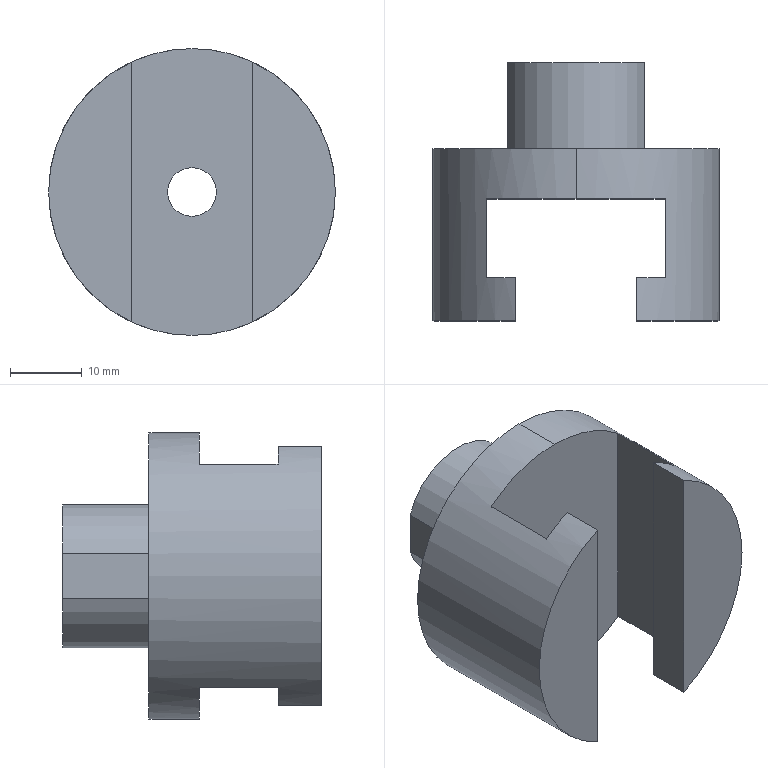Part | STEP file | union head A | 1 solid | 20 faces | box 40 x 36 x 40 mm | volume 19001 mm3 | plane 13 | cylinder 7 | commonest cylinder face diameters 20 x3 6.8 x2 40 x2
STEP:
#1=CARTESIAN_POINT('',(0.,0.,0.));
#2=DIRECTION('',(0.,0.,1.));
#3=DIRECTION('',(1.,0.,0.));
#4=AXIS2_PLACEMENT_3D('',#1,#2,#3);
#5=CARTESIAN_POINT('',(0.,17.,3.4));
#6=VERTEX_POINT('',#5);
#7=CARTESIAN_POINT('',(0.,36.,3.4));
#8=VERTEX_POINT('',#7);
#9=CARTESIAN_POINT('',(0.,36.,3.4));
#10=DIRECTION('',(0.,1.,0.));
#11=VECTOR('',#10,1.);
#12=LINE('',#9,#11);
#13=CARTESIAN_POINT('',(0.,36.,0.));
#14=DIRECTION('',(0.,1.,0.));
#15=DIRECTION('',(0.,0.,1.));
#16=AXIS2_PLACEMENT_3D('',#13,#14,#15);
#17=CYLINDRICAL_SURFACE('',#16,3.4);
#18=CARTESIAN_POINT('',(6.283,0.));
#19=DIRECTION('',(0.,1.));
#20=VECTOR('',#19,1.);
#21=LINE('',#18,#20);
#22=(GEOMETRIC_REPRESENTATION_CONTEXT(2)PARAMETRIC_REPRESENTATION_CONTEXT()REPRESENTATION_CONTEXT('',''));
#23=DEFINITIONAL_REPRESENTATION('',(#21),#22);
#24=PCURVE('',#17,#23);
#25=CARTESIAN_POINT('',(0.,36.,0.));
#26=DIRECTION('',(0.,1.,0.));
#27=DIRECTION('',(0.,0.,1.));
#28=AXIS2_PLACEMENT_3D('',#25,#26,#27);
#29=CYLINDRICAL_SURFACE('',#28,3.4);
#30=CARTESIAN_POINT('',(0.,0.));
#31=DIRECTION('',(0.,1.));
#32=VECTOR('',#31,1.);
#33=LINE('',#30,#32);
#34=(GEOMETRIC_REPRESENTATION_CONTEXT(2)PARAMETRIC_REPRESENTATION_CONTEXT()REPRESENTATION_CONTEXT('',''));
#35=DEFINITIONAL_REPRESENTATION('',(#33),#34);
#36=PCURVE('',#29,#35);
#37=SURFACE_CURVE('',#12,(#24,#36),.PCURVE_S1.);
#38=EDGE_CURVE('',#6,#8,#37,.T.);
#39=ORIENTED_EDGE('',*,*,#38,.T.);
#40=CARTESIAN_POINT('',(0.,36.,-3.4));
#41=VERTEX_POINT('',#40);
#42=CARTESIAN_POINT('',(0.,36.,0.));
#43=DIRECTION('',(0.,1.,0.));
#44=DIRECTION('',(0.,0.,1.));
#45=AXIS2_PLACEMENT_3D('',#42,#43,#44);
#46=CIRCLE('',#45,3.4);
#47=CARTESIAN_POINT('',(0.,0.));
#48=DIRECTION('',(1.,0.));
#49=VECTOR('',#48,1.);
#50=LINE('',#47,#49);
#51=(GEOMETRIC_REPRESENTATION_CONTEXT(2)PARAMETRIC_REPRESENTATION_CONTEXT()REPRESENTATION_CONTEXT('',''));
#52=DEFINITIONAL_REPRESENTATION('',(#50),#51);
#53=PCURVE('',#17,#52);
#54=CARTESIAN_POINT('',(0.,36.,0.));
#55=DIRECTION('',(0.,-1.,0.));
#56=DIRECTION('',(0.,0.,-1.));
#57=AXIS2_PLACEMENT_3D('',#54,#55,#56);
#58=PLANE('',#57);
#59=CARTESIAN_POINT('',(-3.4,0.));
#60=CARTESIAN_POINT('',(-3.4,5.889));
#61=CARTESIAN_POINT('',(1.7,2.944));
#62=CARTESIAN_POINT('',(6.8,0.));
#63=CARTESIAN_POINT('',(1.7,-2.944));
#64=CARTESIAN_POINT('',(-3.4,-5.889));
#65=CARTESIAN_POINT('',(-3.4,0.));
#66=(BOUNDED_CURVE()B_SPLINE_CURVE(2,(#59,#60,#61,#62,#63,#64,#65),.UNSPECIFIED.,.T.,.F.)B_SPLINE_CURVE_WITH_KNOTS((1,2,2,2,2,1),(-2.094,0.,2.094,4.189,6.283,8.378),.UNSPECIFIED.)CURVE()GEOMETRIC_REPRESENTATION_ITEM()RATIONAL_B_SPLINE_CURVE((1.,0.5,1.,0.5,1.,0.5,1.))REPRESENTATION_ITEM(''));
#67=(GEOMETRIC_REPRESENTATION_CONTEXT(2)PARAMETRIC_REPRESENTATION_CONTEXT()REPRESENTATION_CONTEXT('',''));
#68=DEFINITIONAL_REPRESENTATION('',(#66),#67);
#69=PCURVE('',#58,#68);
#70=SURFACE_CURVE('',#46,(#53,#69),.PCURVE_S1.);
#71=EDGE_CURVE('',#41,#8,#70,.T.);
#72=ORIENTED_EDGE('',*,*,#71,.F.);
#73=CARTESIAN_POINT('',(0.,17.,-3.4));
#74=VERTEX_POINT('',#73);
#75=CARTESIAN_POINT('',(0.,36.,-3.4));
#76=DIRECTION('',(0.,1.,0.));
#77=VECTOR('',#76,1.);
#78=LINE('',#75,#77);
#79=CARTESIAN_POINT('',(3.142,0.));
#80=DIRECTION('',(0.,1.));
#81=VECTOR('',#80,1.);
#82=LINE('',#79,#81);
#83=(GEOMETRIC_REPRESENTATION_CONTEXT(2)PARAMETRIC_REPRESENTATION_CONTEXT()REPRESENTATION_CONTEXT('',''));
#84=DEFINITIONAL_REPRESENTATION('',(#82),#83);
#85=PCURVE('',#17,#84);
#86=CARTESIAN_POINT('',(3.142,0.));
#87=DIRECTION('',(0.,1.));
#88=VECTOR('',#87,1.);
#89=LINE('',#86,#88);
#90=(GEOMETRIC_REPRESENTATION_CONTEXT(2)PARAMETRIC_REPRESENTATION_CONTEXT()REPRESENTATION_CONTEXT('',''));
#91=DEFINITIONAL_REPRESENTATION('',(#89),#90);
#92=PCURVE('',#29,#91);
#93=SURFACE_CURVE('',#78,(#85,#92),.PCURVE_S1.);
#94=EDGE_CURVE('',#74,#41,#93,.T.);
#95=ORIENTED_EDGE('',*,*,#94,.F.);
#96=CARTESIAN_POINT('',(0.,17.,0.));
#97=DIRECTION('',(0.,1.,0.));
#98=DIRECTION('',(0.,0.,1.));
#99=AXIS2_PLACEMENT_3D('',#96,#97,#98);
#100=CIRCLE('',#99,3.4);
#101=CARTESIAN_POINT('',(0.,-19.));
#102=DIRECTION('',(1.,0.));
#103=VECTOR('',#102,1.);
#104=LINE('',#101,#103);
#105=(GEOMETRIC_REPRESENTATION_CONTEXT(2)PARAMETRIC_REPRESENTATION_CONTEXT()REPRESENTATION_CONTEXT('',''));
#106=DEFINITIONAL_REPRESENTATION('',(#104),#105);
#107=PCURVE('',#17,#106);
#108=CARTESIAN_POINT('',(-12.5,17.,-20.));
#109=DIRECTION('',(0.,1.,0.));
#110=DIRECTION('',(0.,0.,1.));
#111=AXIS2_PLACEMENT_3D('',#108,#109,#110);
#112=PLANE('',#111);
#113=CARTESIAN_POINT('',(20.,12.5));
#114=DIRECTION('',(1.,0.));
#115=AXIS2_PLACEMENT_2D('',#113,#114);
#116=CIRCLE('',#115,3.4);
#117=(GEOMETRIC_REPRESENTATION_CONTEXT(2)PARAMETRIC_REPRESENTATION_CONTEXT()REPRESENTATION_CONTEXT('',''));
#118=DEFINITIONAL_REPRESENTATION('',(#116),#117);
#119=PCURVE('',#112,#118);
#120=SURFACE_CURVE('',#100,(#107,#119),.PCURVE_S1.);
#121=EDGE_CURVE('',#74,#6,#120,.T.);
#122=ORIENTED_EDGE('',*,*,#121,.T.);
#123=EDGE_LOOP('',(#39,#72,#95,#122));
#124=FACE_BOUND('',#123,.F.);
#125=ADVANCED_FACE('',(#124),#17,.F.);
#126=CARTESIAN_POINT('',(0.,24.,-20.));
#127=VERTEX_POINT('',#126);
#128=CARTESIAN_POINT('',(0.,24.,20.));
#129=VERTEX_POINT('',#128);
#130=CARTESIAN_POINT('',(0.,24.,0.));
#131=DIRECTION('',(0.,-1.,0.));
#132=DIRECTION('',(0.,0.,-1.));
#133=AXIS2_PLACEMENT_3D('',#130,#131,#132);
#134=CIRCLE('',#133,20.);
#135=CARTESIAN_POINT('',(0.,0.,0.));
#136=DIRECTION('',(0.,-1.,0.));
#137=DIRECTION('',(0.,0.,-1.));
#138=AXIS2_PLACEMENT_3D('',#135,#136,#137);
#139=CYLINDRICAL_SURFACE('',#138,20.);
#140=CARTESIAN_POINT('',(0.,-24.));
#141=DIRECTION('',(1.,0.));
#142=VECTOR('',#141,1.);
#143=LINE('',#140,#142);
#144=(GEOMETRIC_REPRESENTATION_CONTEXT(2)PARAMETRIC_REPRESENTATION_CONTEXT()REPRESENTATION_CONTEXT('',''));
#145=DEFINITIONAL_REPRESENTATION('',(#143),#144);
#146=PCURVE('',#139,#145);
#147=CARTESIAN_POINT('',(-10.,24.,0.));
#148=DIRECTION('',(0.,-1.,0.));
#149=DIRECTION('',(0.,0.,-1.));
#150=AXIS2_PLACEMENT_3D('',#147,#148,#149);
#151=PLANE('',#150);
#152=CARTESIAN_POINT('',(0.,10.));
#153=DIRECTION('',(1.,0.));
#154=AXIS2_PLACEMENT_2D('',#152,#153);
#155=CIRCLE('',#154,20.);
#156=(GEOMETRIC_REPRESENTATION_CONTEXT(2)PARAMETRIC_REPRESENTATION_CONTEXT()REPRESENTATION_CONTEXT('',''));
#157=DEFINITIONAL_REPRESENTATION('',(#155),#156);
#158=PCURVE('',#151,#157);
#159=SURFACE_CURVE('',#134,(#146,#158),.PCURVE_S1.);
#160=EDGE_CURVE('',#127,#129,#159,.T.);
#161=ORIENTED_EDGE('',*,*,#160,.T.);
#162=CARTESIAN_POINT('',(0.,17.,20.));
#163=VERTEX_POINT('',#162);
#164=CARTESIAN_POINT('',(0.,0.,20.));
#165=DIRECTION('',(0.,-1.,0.));
#166=VECTOR('',#165,1.);
#167=LINE('',#164,#166);
#168=CARTESIAN_POINT('',(3.142,0.));
#169=DIRECTION('',(0.,1.));
#170=VECTOR('',#169,1.);
#171=LINE('',#168,#170);
#172=(GEOMETRIC_REPRESENTATION_CONTEXT(2)PARAMETRIC_REPRESENTATION_CONTEXT()REPRESENTATION_CONTEXT('',''));
#173=DEFINITIONAL_REPRESENTATION('',(#171),#172);
#174=PCURVE('',#139,#173);
#175=CARTESIAN_POINT('',(0.,0.,0.));
#176=DIRECTION('',(0.,-1.,0.));
#177=DIRECTION('',(0.,0.,-1.));
#178=AXIS2_PLACEMENT_3D('',#175,#176,#177);
#179=CYLINDRICAL_SURFACE('',#178,20.);
#180=CARTESIAN_POINT('',(3.142,0.));
#181=DIRECTION('',(0.,1.));
#182=VECTOR('',#181,1.);
#183=LINE('',#180,#182);
#184=(GEOMETRIC_REPRESENTATION_CONTEXT(2)PARAMETRIC_REPRESENTATION_CONTEXT()REPRESENTATION_CONTEXT('',''));
#185=DEFINITIONAL_REPRESENTATION('',(#183),#184);
#186=PCURVE('',#179,#185);
#187=SURFACE_CURVE('',#167,(#174,#186),.PCURVE_S1.);
#188=EDGE_CURVE('',#129,#163,#187,.T.);
#189=ORIENTED_EDGE('',*,*,#188,.T.);
#190=CARTESIAN_POINT('',(12.5,17.,15.612));
#191=VERTEX_POINT('',#190);
#192=CARTESIAN_POINT('',(0.,17.,0.));
#193=DIRECTION('',(0.,1.,0.));
#194=DIRECTION('',(0.,0.,1.));
#195=AXIS2_PLACEMENT_3D('',#192,#193,#194);
#196=CIRCLE('',#195,20.);
#197=CARTESIAN_POINT('',(3.142,-17.));
#198=DIRECTION('',(-1.,0.));
#199=VECTOR('',#198,1.);
#200=LINE('',#197,#199);
#201=(GEOMETRIC_REPRESENTATION_CONTEXT(2)PARAMETRIC_REPRESENTATION_CONTEXT()REPRESENTATION_CONTEXT('',''));
#202=DEFINITIONAL_REPRESENTATION('',(#200),#201);
#203=PCURVE('',#139,#202);
#204=CARTESIAN_POINT('',(20.,12.5));
#205=DIRECTION('',(1.,0.));
#206=AXIS2_PLACEMENT_2D('',#204,#205);
#207=CIRCLE('',#206,20.);
#208=(GEOMETRIC_REPRESENTATION_CONTEXT(2)PARAMETRIC_REPRESENTATION_CONTEXT()REPRESENTATION_CONTEXT('',''));
#209=DEFINITIONAL_REPRESENTATION('',(#207),#208);
#210=PCURVE('',#112,#209);
#211=SURFACE_CURVE('',#196,(#203,#210),.PCURVE_S1.);
#212=EDGE_CURVE('',#163,#191,#211,.T.);
#213=ORIENTED_EDGE('',*,*,#212,.T.);
#214=CARTESIAN_POINT('',(12.5,6.,15.612));
#215=VERTEX_POINT('',#214);
#216=CARTESIAN_POINT('',(12.5,0.,15.612));
#217=DIRECTION('',(0.,-1.,0.));
#218=VECTOR('',#217,1.);
#219=LINE('',#216,#218);
#220=CARTESIAN_POINT('',(2.466,0.));
#221=DIRECTION('',(0.,1.));
#222=VECTOR('',#221,1.);
#223=LINE('',#220,#222);
#224=(GEOMETRIC_REPRESENTATION_CONTEXT(2)PARAMETRIC_REPRESENTATION_CONTEXT()REPRESENTATION_CONTEXT('',''));
#225=DEFINITIONAL_REPRESENTATION('',(#223),#224);
#226=PCURVE('',#139,#225);
#227=CARTESIAN_POINT('',(12.5,17.,-20.));
#228=DIRECTION('',(1.,0.,0.));
#229=DIRECTION('',(0.,1.,0.));
#230=AXIS2_PLACEMENT_3D('',#227,#228,#229);
#231=PLANE('',#230);
#232=CARTESIAN_POINT('',(-17.,35.612));
#233=DIRECTION('',(-1.,0.));
#234=VECTOR('',#233,1.);
#235=LINE('',#232,#234);
#236=(GEOMETRIC_REPRESENTATION_CONTEXT(2)PARAMETRIC_REPRESENTATION_CONTEXT()REPRESENTATION_CONTEXT('',''));
#237=DEFINITIONAL_REPRESENTATION('',(#235),#236);
#238=PCURVE('',#231,#237);
#239=SURFACE_CURVE('',#219,(#226,#238),.PCURVE_S1.);
#240=EDGE_CURVE('',#191,#215,#239,.T.);
#241=ORIENTED_EDGE('',*,*,#240,.T.);
#242=CARTESIAN_POINT('',(8.5,6.,18.104));
#243=VERTEX_POINT('',#242);
#244=CARTESIAN_POINT('',(0.,6.,0.));
#245=DIRECTION('',(0.,-1.,0.));
#246=DIRECTION('',(0.,0.,-1.));
#247=AXIS2_PLACEMENT_3D('',#244,#245,#246);
#248=CIRCLE('',#247,20.);
#249=CARTESIAN_POINT('',(0.,-6.));
#250=DIRECTION('',(1.,0.));
#251=VECTOR('',#250,1.);
#252=LINE('',#249,#251);
#253=(GEOMETRIC_REPRESENTATION_CONTEXT(2)PARAMETRIC_REPRESENTATION_CONTEXT()REPRESENTATION_CONTEXT('',''));
#254=DEFINITIONAL_REPRESENTATION('',(#252),#253);
#255=PCURVE('',#139,#254);
#256=CARTESIAN_POINT('',(8.5,6.,-20.));
#257=DIRECTION('',(0.,-1.,0.));
#258=DIRECTION('',(0.,0.,-1.));
#259=AXIS2_PLACEMENT_3D('',#256,#257,#258);
#260=PLANE('',#259);
#261=CARTESIAN_POINT('',(-20.,-8.5));
#262=DIRECTION('',(1.,0.));
#263=AXIS2_PLACEMENT_2D('',#261,#262);
#264=CIRCLE('',#263,20.);
#265=(GEOMETRIC_REPRESENTATION_CONTEXT(2)PARAMETRIC_REPRESENTATION_CONTEXT()REPRESENTATION_CONTEXT('',''));
#266=DEFINITIONAL_REPRESENTATION('',(#264),#265);
#267=PCURVE('',#260,#266);
#268=SURFACE_CURVE('',#248,(#255,#267),.PCURVE_S1.);
#269=EDGE_CURVE('',#215,#243,#268,.T.);
#270=ORIENTED_EDGE('',*,*,#269,.T.);
#271=CARTESIAN_POINT('',(8.5,0.,18.104));
#272=VERTEX_POINT('',#271);
#273=CARTESIAN_POINT('',(8.5,0.,18.104));
#274=DIRECTION('',(0.,-1.,0.));
#275=VECTOR('',#274,1.);
#276=LINE('',#273,#275);
#277=CARTESIAN_POINT('',(2.703,0.));
#278=DIRECTION('',(0.,1.));
#279=VECTOR('',#278,1.);
#280=LINE('',#277,#279);
#281=(GEOMETRIC_REPRESENTATION_CONTEXT(2)PARAMETRIC_REPRESENTATION_CONTEXT()REPRESENTATION_CONTEXT('',''));
#282=DEFINITIONAL_REPRESENTATION('',(#280),#281);
#283=PCURVE('',#139,#282);
#284=CARTESIAN_POINT('',(8.5,0.,-20.));
#285=DIRECTION('',(1.,0.,0.));
#286=DIRECTION('',(0.,0.,-1.));
#287=AXIS2_PLACEMENT_3D('',#284,#285,#286);
#288=PLANE('',#287);
#289=CARTESIAN_POINT('',(-38.104,0.));
#290=DIRECTION('',(0.,-1.));
#291=VECTOR('',#290,1.);
#292=LINE('',#289,#291);
#293=(GEOMETRIC_REPRESENTATION_CONTEXT(2)PARAMETRIC_REPRESENTATION_CONTEXT()REPRESENTATION_CONTEXT('',''));
#294=DEFINITIONAL_REPRESENTATION('',(#292),#293);
#295=PCURVE('',#288,#294);
#296=SURFACE_CURVE('',#276,(#283,#295),.PCURVE_S1.);
#297=EDGE_CURVE('',#243,#272,#296,.T.);
#298=ORIENTED_EDGE('',*,*,#297,.T.);
#299=CARTESIAN_POINT('',(8.5,0.,-18.104));
#300=VERTEX_POINT('',#299);
#301=CARTESIAN_POINT('',(0.,0.,0.));
#302=DIRECTION('',(0.,-1.,0.));
#303=DIRECTION('',(0.,0.,-1.));
#304=AXIS2_PLACEMENT_3D('',#301,#302,#303);
#305=CIRCLE('',#304,20.);
#306=CARTESIAN_POINT('',(0.,0.));
#307=DIRECTION('',(1.,0.));
#308=VECTOR('',#307,1.);
#309=LINE('',#306,#308);
#310=(GEOMETRIC_REPRESENTATION_CONTEXT(2)PARAMETRIC_REPRESENTATION_CONTEXT()REPRESENTATION_CONTEXT('',''));
#311=DEFINITIONAL_REPRESENTATION('',(#309),#310);
#312=PCURVE('',#139,#311);
#313=CARTESIAN_POINT('',(-20.,0.,0.));
#314=DIRECTION('',(0.,1.,0.));
#315=DIRECTION('',(0.,0.,1.));
#316=AXIS2_PLACEMENT_3D('',#313,#314,#315);
#317=PLANE('',#316);
#318=CARTESIAN_POINT('',(-20.,20.));
#319=CARTESIAN_POINT('',(-20.,54.641));
#320=CARTESIAN_POINT('',(10.,37.321));
#321=CARTESIAN_POINT('',(40.,20.));
#322=CARTESIAN_POINT('',(10.,2.679));
#323=CARTESIAN_POINT('',(-20.,-14.641));
#324=CARTESIAN_POINT('',(-20.,20.));
#325=(BOUNDED_CURVE()B_SPLINE_CURVE(2,(#318,#319,#320,#321,#322,#323,#324),.UNSPECIFIED.,.T.,.F.)B_SPLINE_CURVE_WITH_KNOTS((1,2,2,2,2,1),(-2.094,0.,2.094,4.189,6.283,8.378),.UNSPECIFIED.)CURVE()GEOMETRIC_REPRESENTATION_ITEM()RATIONAL_B_SPLINE_CURVE((1.,0.5,1.,0.5,1.,0.5,1.))REPRESENTATION_ITEM(''));
#326=(GEOMETRIC_REPRESENTATION_CONTEXT(2)PARAMETRIC_REPRESENTATION_CONTEXT()REPRESENTATION_CONTEXT('',''));
#327=DEFINITIONAL_REPRESENTATION('',(#325),#326);
#328=PCURVE('',#317,#327);
#329=SURFACE_CURVE('',#305,(#312,#328),.PCURVE_S1.);
#330=EDGE_CURVE('',#300,#272,#329,.T.);
#331=ORIENTED_EDGE('',*,*,#330,.F.);
#332=CARTESIAN_POINT('',(8.5,6.,-18.104));
#333=VERTEX_POINT('',#332);
#334=CARTESIAN_POINT('',(8.5,0.,-18.104));
#335=DIRECTION('',(0.,1.,0.));
#336=VECTOR('',#335,1.);
#337=LINE('',#334,#336);
#338=CARTESIAN_POINT('',(0.439,0.));
#339=DIRECTION('',(0.,-1.));
#340=VECTOR('',#339,1.);
#341=LINE('',#338,#340);
#342=(GEOMETRIC_REPRESENTATION_CONTEXT(2)PARAMETRIC_REPRESENTATION_CONTEXT()REPRESENTATION_CONTEXT('',''));
#343=DEFINITIONAL_REPRESENTATION('',(#341),#342);
#344=PCURVE('',#139,#343);
#345=CARTESIAN_POINT('',(-1.896,0.));
#346=DIRECTION('',(0.,1.));
#347=VECTOR('',#346,1.);
#348=LINE('',#345,#347);
#349=(GEOMETRIC_REPRESENTATION_CONTEXT(2)PARAMETRIC_REPRESENTATION_CONTEXT()REPRESENTATION_CONTEXT('',''));
#350=DEFINITIONAL_REPRESENTATION('',(#348),#349);
#351=PCURVE('',#288,#350);
#352=SURFACE_CURVE('',#337,(#344,#351),.PCURVE_S1.);
#353=EDGE_CURVE('',#300,#333,#352,.T.);
#354=ORIENTED_EDGE('',*,*,#353,.T.);
#355=CARTESIAN_POINT('',(12.5,6.,-15.612));
#356=VERTEX_POINT('',#355);
#357=CARTESIAN_POINT('',(0.,6.,0.));
#358=DIRECTION('',(0.,-1.,0.));
#359=DIRECTION('',(0.,0.,-1.));
#360=AXIS2_PLACEMENT_3D('',#357,#358,#359);
#361=CIRCLE('',#360,20.);
#362=CARTESIAN_POINT('',(0.,-6.));
#363=DIRECTION('',(1.,0.));
#364=VECTOR('',#363,1.);
#365=LINE('',#362,#364);
#366=(GEOMETRIC_REPRESENTATION_CONTEXT(2)PARAMETRIC_REPRESENTATION_CONTEXT()REPRESENTATION_CONTEXT('',''));
#367=DEFINITIONAL_REPRESENTATION('',(#365),#366);
#368=PCURVE('',#139,#367);
#369=CARTESIAN_POINT('',(-20.,-8.5));
#370=DIRECTION('',(1.,0.));
#371=AXIS2_PLACEMENT_2D('',#369,#370);
#372=CIRCLE('',#371,20.);
#373=(GEOMETRIC_REPRESENTATION_CONTEXT(2)PARAMETRIC_REPRESENTATION_CONTEXT()REPRESENTATION_CONTEXT('',''));
#374=DEFINITIONAL_REPRESENTATION('',(#372),#373);
#375=PCURVE('',#260,#374);
#376=SURFACE_CURVE('',#361,(#368,#375),.PCURVE_S1.);
#377=EDGE_CURVE('',#333,#356,#376,.T.);
#378=ORIENTED_EDGE('',*,*,#377,.T.);
#379=CARTESIAN_POINT('',(12.5,17.,-15.612));
#380=VERTEX_POINT('',#379);
#381=CARTESIAN_POINT('',(12.5,0.,-15.612));
#382=DIRECTION('',(0.,1.,0.));
#383=VECTOR('',#382,1.);
#384=LINE('',#381,#383);
#385=CARTESIAN_POINT('',(0.6751,0.));
#386=DIRECTION('',(0.,-1.));
#387=VECTOR('',#386,1.);
#388=LINE('',#385,#387);
#389=(GEOMETRIC_REPRESENTATION_CONTEXT(2)PARAMETRIC_REPRESENTATION_CONTEXT()REPRESENTATION_CONTEXT('',''));
#390=DEFINITIONAL_REPRESENTATION('',(#388),#389);
#391=PCURVE('',#139,#390);
#392=CARTESIAN_POINT('',(-17.,4.388));
#393=DIRECTION('',(1.,0.));
#394=VECTOR('',#393,1.);
#395=LINE('',#392,#394);
#396=(GEOMETRIC_REPRESENTATION_CONTEXT(2)PARAMETRIC_REPRESENTATION_CONTEXT()REPRESENTATION_CONTEXT('',''));
#397=DEFINITIONAL_REPRESENTATION('',(#395),#396);
#398=PCURVE('',#231,#397);
#399=SURFACE_CURVE('',#384,(#391,#398),.PCURVE_S1.);
#400=EDGE_CURVE('',#356,#380,#399,.T.);
#401=ORIENTED_EDGE('',*,*,#400,.T.);
#402=CARTESIAN_POINT('',(0.,17.,-20.));
#403=VERTEX_POINT('',#402);
#404=CARTESIAN_POINT('',(0.,17.,0.));
#405=DIRECTION('',(0.,1.,0.));
#406=DIRECTION('',(0.,0.,1.));
#407=AXIS2_PLACEMENT_3D('',#404,#405,#406);
#408=CIRCLE('',#407,20.);
#409=CARTESIAN_POINT('',(3.142,-17.));
#410=DIRECTION('',(-1.,0.));
#411=VECTOR('',#410,1.);
#412=LINE('',#409,#411);
#413=(GEOMETRIC_REPRESENTATION_CONTEXT(2)PARAMETRIC_REPRESENTATION_CONTEXT()REPRESENTATION_CONTEXT('',''));
#414=DEFINITIONAL_REPRESENTATION('',(#412),#413);
#415=PCURVE('',#139,#414);
#416=CARTESIAN_POINT('',(20.,12.5));
#417=DIRECTION('',(1.,0.));
#418=AXIS2_PLACEMENT_2D('',#416,#417);
#419=CIRCLE('',#418,20.);
#420=(GEOMETRIC_REPRESENTATION_CONTEXT(2)PARAMETRIC_REPRESENTATION_CONTEXT()REPRESENTATION_CONTEXT('',''));
#421=DEFINITIONAL_REPRESENTATION('',(#419),#420);
#422=PCURVE('',#112,#421);
#423=SURFACE_CURVE('',#408,(#415,#422),.PCURVE_S1.);
#424=EDGE_CURVE('',#380,#403,#423,.T.);
#425=ORIENTED_EDGE('',*,*,#424,.T.);
#426=CARTESIAN_POINT('',(0.,0.,-20.));
#427=DIRECTION('',(0.,-1.,0.));
#428=VECTOR('',#427,1.);
#429=LINE('',#426,#428);
#430=CARTESIAN_POINT('',(0.,0.));
#431=DIRECTION('',(0.,1.));
#432=VECTOR('',#431,1.);
#433=LINE('',#430,#432);
#434=(GEOMETRIC_REPRESENTATION_CONTEXT(2)PARAMETRIC_REPRESENTATION_CONTEXT()REPRESENTATION_CONTEXT('',''));
#435=DEFINITIONAL_REPRESENTATION('',(#433),#434);
#436=PCURVE('',#139,#435);
#437=CARTESIAN_POINT('',(6.283,0.));
#438=DIRECTION('',(0.,1.));
#439=VECTOR('',#438,1.);
#440=LINE('',#437,#439);
#441=(GEOMETRIC_REPRESENTATION_CONTEXT(2)PARAMETRIC_REPRESENTATION_CONTEXT()REPRESENTATION_CONTEXT('',''));
#442=DEFINITIONAL_REPRESENTATION('',(#440),#441);
#443=PCURVE('',#179,#442);
#444=SURFACE_CURVE('',#429,(#436,#443),.PCURVE_S1.);
#445=EDGE_CURVE('',#127,#403,#444,.T.);
#446=ORIENTED_EDGE('',*,*,#445,.F.);
#447=EDGE_LOOP('',(#161,#189,#213,#241,#270,#298,#331,#354,#378,#401,#425,#446));
#448=FACE_BOUND('',#447,.T.);
#449=ADVANCED_FACE('',(#448),#139,.T.);
#450=CARTESIAN_POINT('',(-9.5,36.,-3.122));
#451=VERTEX_POINT('',#450);
#452=CARTESIAN_POINT('',(0.,36.,-10.));
#453=VERTEX_POINT('',#452);
#454=CARTESIAN_POINT('',(0.,36.,0.));
#455=DIRECTION('',(0.,-1.,0.));
#456=DIRECTION('',(0.,0.,-1.));
#457=AXIS2_PLACEMENT_3D('',#454,#455,#456);
#458=CIRCLE('',#457,10.);
#459=CARTESIAN_POINT('',(0.,0.,0.));
#460=DIRECTION('',(0.,-1.,0.));
#461=DIRECTION('',(0.,0.,-1.));
#462=AXIS2_PLACEMENT_3D('',#459,#460,#461);
#463=CYLINDRICAL_SURFACE('',#462,10.);
#464=CARTESIAN_POINT('',(0.,-36.));
#465=DIRECTION('',(1.,0.));
#466=VECTOR('',#465,1.);
#467=LINE('',#464,#466);
#468=(GEOMETRIC_REPRESENTATION_CONTEXT(2)PARAMETRIC_REPRESENTATION_CONTEXT()REPRESENTATION_CONTEXT('',''));
#469=DEFINITIONAL_REPRESENTATION('',(#467),#468);
#470=PCURVE('',#463,#469);
#471=CARTESIAN_POINT('',(0.,0.));
#472=DIRECTION('',(1.,0.));
#473=AXIS2_PLACEMENT_2D('',#471,#472);
#474=CIRCLE('',#473,10.);
#475=(GEOMETRIC_REPRESENTATION_CONTEXT(2)PARAMETRIC_REPRESENTATION_CONTEXT()REPRESENTATION_CONTEXT('',''));
#476=DEFINITIONAL_REPRESENTATION('',(#474),#475);
#477=PCURVE('',#58,#476);
#478=SURFACE_CURVE('',#458,(#470,#477),.PCURVE_S1.);
#479=EDGE_CURVE('',#451,#453,#478,.T.);
#480=ORIENTED_EDGE('',*,*,#479,.T.);
#481=CARTESIAN_POINT('',(0.,24.,-10.));
#482=VERTEX_POINT('',#481);
#483=CARTESIAN_POINT('',(0.,0.,-10.));
#484=DIRECTION('',(0.,-1.,0.));
#485=VECTOR('',#484,1.);
#486=LINE('',#483,#485);
#487=CARTESIAN_POINT('',(6.283,0.));
#488=DIRECTION('',(0.,1.));
#489=VECTOR('',#488,1.);
#490=LINE('',#487,#489);
#491=(GEOMETRIC_REPRESENTATION_CONTEXT(2)PARAMETRIC_REPRESENTATION_CONTEXT()REPRESENTATION_CONTEXT('',''));
#492=DEFINITIONAL_REPRESENTATION('',(#490),#491);
#493=PCURVE('',#463,#492);
#494=CARTESIAN_POINT('',(0.,0.,0.));
#495=DIRECTION('',(0.,-1.,0.));
#496=DIRECTION('',(0.,0.,-1.));
#497=AXIS2_PLACEMENT_3D('',#494,#495,#496);
#498=CYLINDRICAL_SURFACE('',#497,10.);
#499=CARTESIAN_POINT('',(0.,0.));
#500=DIRECTION('',(0.,1.));
#501=VECTOR('',#500,1.);
#502=LINE('',#499,#501);
#503=(GEOMETRIC_REPRESENTATION_CONTEXT(2)PARAMETRIC_REPRESENTATION_CONTEXT()REPRESENTATION_CONTEXT('',''));
#504=DEFINITIONAL_REPRESENTATION('',(#502),#503);
#505=PCURVE('',#498,#504);
#506=SURFACE_CURVE('',#486,(#493,#505),.PCURVE_S1.);
#507=EDGE_CURVE('',#453,#482,#506,.T.);
#508=ORIENTED_EDGE('',*,*,#507,.T.);
#509=CARTESIAN_POINT('',(-9.5,24.,-3.122));
#510=VERTEX_POINT('',#509);
#511=CARTESIAN_POINT('',(0.,24.,0.));
#512=DIRECTION('',(0.,-1.,0.));
#513=DIRECTION('',(0.,0.,-1.));
#514=AXIS2_PLACEMENT_3D('',#511,#512,#513);
#515=CIRCLE('',#514,10.);
#516=CARTESIAN_POINT('',(0.,-24.));
#517=DIRECTION('',(1.,0.));
#518=VECTOR('',#517,1.);
#519=LINE('',#516,#518);
#520=(GEOMETRIC_REPRESENTATION_CONTEXT(2)PARAMETRIC_REPRESENTATION_CONTEXT()REPRESENTATION_CONTEXT('',''));
#521=DEFINITIONAL_REPRESENTATION('',(#519),#520);
#522=PCURVE('',#463,#521);
#523=CARTESIAN_POINT('',(0.,10.));
#524=DIRECTION('',(1.,0.));
#525=AXIS2_PLACEMENT_2D('',#523,#524);
#526=CIRCLE('',#525,10.);
#527=(GEOMETRIC_REPRESENTATION_CONTEXT(2)PARAMETRIC_REPRESENTATION_CONTEXT()REPRESENTATION_CONTEXT('',''));
#528=DEFINITIONAL_REPRESENTATION('',(#526),#527);
#529=PCURVE('',#151,#528);
#530=SURFACE_CURVE('',#515,(#522,#529),.PCURVE_S1.);
#531=EDGE_CURVE('',#510,#482,#530,.T.);
#532=ORIENTED_EDGE('',*,*,#531,.F.);
#533=CARTESIAN_POINT('',(-9.5,0.,-3.122));
#534=DIRECTION('',(0.,1.,0.));
#535=VECTOR('',#534,1.);
#536=LINE('',#533,#535);
#537=CARTESIAN_POINT('',(5.03,0.));
#538=DIRECTION('',(0.,-1.));
#539=VECTOR('',#538,1.);
#540=LINE('',#537,#539);
#541=(GEOMETRIC_REPRESENTATION_CONTEXT(2)PARAMETRIC_REPRESENTATION_CONTEXT()REPRESENTATION_CONTEXT('',''));
#542=DEFINITIONAL_REPRESENTATION('',(#540),#541);
#543=PCURVE('',#463,#542);
#544=CARTESIAN_POINT('',(-9.5,6.26,-6.601));
#545=DIRECTION('',(1.,0.,0.));
#546=DIRECTION('',(0.,0.,-1.));
#547=AXIS2_PLACEMENT_3D('',#544,#545,#546);
#548=PLANE('',#547);
#549=CARTESIAN_POINT('',(-3.479,-6.26));
#550=DIRECTION('',(0.,1.));
#551=VECTOR('',#550,1.);
#552=LINE('',#549,#551);
#553=(GEOMETRIC_REPRESENTATION_CONTEXT(2)PARAMETRIC_REPRESENTATION_CONTEXT()REPRESENTATION_CONTEXT('',''));
#554=DEFINITIONAL_REPRESENTATION('',(#552),#553);
#555=PCURVE('',#548,#554);
#556=SURFACE_CURVE('',#536,(#543,#555),.PCURVE_S1.);
#557=EDGE_CURVE('',#510,#451,#556,.T.);
#558=ORIENTED_EDGE('',*,*,#557,.T.);
#559=EDGE_LOOP('',(#480,#508,#532,#558));
#560=FACE_BOUND('',#559,.T.);
#561=ADVANCED_FACE('',(#560),#463,.T.);
#562=CARTESIAN_POINT('',(-8.5,0.,18.104));
#563=VERTEX_POINT('',#562);
#564=CARTESIAN_POINT('',(-8.5,0.,-18.104));
#565=VERTEX_POINT('',#564);
#566=CARTESIAN_POINT('',(0.,0.,0.));
#567=DIRECTION('',(0.,-1.,0.));
#568=DIRECTION('',(0.,0.,-1.));
#569=AXIS2_PLACEMENT_3D('',#566,#567,#568);
#570=CIRCLE('',#569,20.);
#571=CARTESIAN_POINT('',(-20.,0.,0.));
#572=DIRECTION('',(0.,1.,0.));
#573=DIRECTION('',(0.,0.,1.));
#574=AXIS2_PLACEMENT_3D('',#571,#572,#573);
#575=PLANE('',#574);
#576=CARTESIAN_POINT('',(-20.,20.));
#577=CARTESIAN_POINT('',(-20.,54.641));
#578=CARTESIAN_POINT('',(10.,37.321));
#579=CARTESIAN_POINT('',(40.,20.));
#580=CARTESIAN_POINT('',(10.,2.679));
#581=CARTESIAN_POINT('',(-20.,-14.641));
#582=CARTESIAN_POINT('',(-20.,20.));
#583=(BOUNDED_CURVE()B_SPLINE_CURVE(2,(#576,#577,#578,#579,#580,#581,#582),.UNSPECIFIED.,.T.,.F.)B_SPLINE_CURVE_WITH_KNOTS((1,2,2,2,2,1),(-2.094,0.,2.094,4.189,6.283,8.378),.UNSPECIFIED.)CURVE()GEOMETRIC_REPRESENTATION_ITEM()RATIONAL_B_SPLINE_CURVE((1.,0.5,1.,0.5,1.,0.5,1.))REPRESENTATION_ITEM(''));
#584=(GEOMETRIC_REPRESENTATION_CONTEXT(2)PARAMETRIC_REPRESENTATION_CONTEXT()REPRESENTATION_CONTEXT('',''));
#585=DEFINITIONAL_REPRESENTATION('',(#583),#584);
#586=PCURVE('',#575,#585);
#587=CARTESIAN_POINT('',(0.,0.));
#588=DIRECTION('',(1.,0.));
#589=VECTOR('',#588,1.);
#590=LINE('',#587,#589);
#591=(GEOMETRIC_REPRESENTATION_CONTEXT(2)PARAMETRIC_REPRESENTATION_CONTEXT()REPRESENTATION_CONTEXT('',''));
#592=DEFINITIONAL_REPRESENTATION('',(#590),#591);
#593=PCURVE('',#179,#592);
#594=SURFACE_CURVE('',#570,(#586,#593),.PCURVE_S1.);
#595=EDGE_CURVE('',#563,#565,#594,.T.);
#596=ORIENTED_EDGE('',*,*,#595,.T.);
#597=CARTESIAN_POINT('',(-8.5,0.,0.));
#598=DIRECTION('',(0.,0.,1.));
#599=VECTOR('',#598,1.);
#600=LINE('',#597,#599);
#601=CARTESIAN_POINT('',(0.,11.5));
#602=DIRECTION('',(1.,0.));
#603=VECTOR('',#602,1.);
#604=LINE('',#601,#603);
#605=(GEOMETRIC_REPRESENTATION_CONTEXT(2)PARAMETRIC_REPRESENTATION_CONTEXT()REPRESENTATION_CONTEXT('',''));
#606=DEFINITIONAL_REPRESENTATION('',(#604),#605);
#607=PCURVE('',#575,#606);
#608=CARTESIAN_POINT('',(-8.5,0.,-20.));
#609=DIRECTION('',(-1.,0.,0.));
#610=DIRECTION('',(0.,0.,1.));
#611=AXIS2_PLACEMENT_3D('',#608,#609,#610);
#612=PLANE('',#611);
#613=CARTESIAN_POINT('',(20.,0.));
#614=DIRECTION('',(1.,0.));
#615=VECTOR('',#614,1.);
#616=LINE('',#613,#615);
#617=(GEOMETRIC_REPRESENTATION_CONTEXT(2)PARAMETRIC_REPRESENTATION_CONTEXT()REPRESENTATION_CONTEXT('',''));
#618=DEFINITIONAL_REPRESENTATION('',(#616),#617);
#619=PCURVE('',#612,#618);
#620=SURFACE_CURVE('',#600,(#607,#619),.PCURVE_S1.);
#621=EDGE_CURVE('',#565,#563,#620,.T.);
#622=ORIENTED_EDGE('',*,*,#621,.T.);
#623=EDGE_LOOP('',(#596,#622));
#624=FACE_BOUND('',#623,.T.);
#625=ADVANCED_FACE('',(#624),#575,.F.);
#626=ORIENTED_EDGE('',*,*,#507,.F.);
#627=CARTESIAN_POINT('',(9.5,36.,-3.122));
#628=VERTEX_POINT('',#627);
#629=CARTESIAN_POINT('',(0.,36.,0.));
#630=DIRECTION('',(0.,-1.,0.));
#631=DIRECTION('',(0.,0.,-1.));
#632=AXIS2_PLACEMENT_3D('',#629,#630,#631);
#633=CIRCLE('',#632,10.);
#634=CARTESIAN_POINT('',(0.,-36.));
#635=DIRECTION('',(1.,0.));
#636=VECTOR('',#635,1.);
#637=LINE('',#634,#636);
#638=(GEOMETRIC_REPRESENTATION_CONTEXT(2)PARAMETRIC_REPRESENTATION_CONTEXT()REPRESENTATION_CONTEXT('',''));
#639=DEFINITIONAL_REPRESENTATION('',(#637),#638);
#640=PCURVE('',#498,#639);
#641=CARTESIAN_POINT('',(0.,0.));
#642=DIRECTION('',(1.,0.));
#643=AXIS2_PLACEMENT_2D('',#641,#642);
#644=CIRCLE('',#643,10.);
#645=(GEOMETRIC_REPRESENTATION_CONTEXT(2)PARAMETRIC_REPRESENTATION_CONTEXT()REPRESENTATION_CONTEXT('',''));
#646=DEFINITIONAL_REPRESENTATION('',(#644),#645);
#647=PCURVE('',#58,#646);
#648=SURFACE_CURVE('',#633,(#640,#647),.PCURVE_S1.);
#649=EDGE_CURVE('',#453,#628,#648,.T.);
#650=ORIENTED_EDGE('',*,*,#649,.T.);
#651=CARTESIAN_POINT('',(9.5,24.,-3.122));
#652=VERTEX_POINT('',#651);
#653=CARTESIAN_POINT('',(9.5,0.,-3.122));
#654=DIRECTION('',(0.,-1.,0.));
#655=VECTOR('',#654,1.);
#656=LINE('',#653,#655);
#657=CARTESIAN_POINT('',(1.253,0.));
#658=DIRECTION('',(0.,1.));
#659=VECTOR('',#658,1.);
#660=LINE('',#657,#659);
#661=(GEOMETRIC_REPRESENTATION_CONTEXT(2)PARAMETRIC_REPRESENTATION_CONTEXT()REPRESENTATION_CONTEXT('',''));
#662=DEFINITIONAL_REPRESENTATION('',(#660),#661);
#663=PCURVE('',#498,#662);
#664=CARTESIAN_POINT('',(9.5,6.26,-9.315));
#665=DIRECTION('',(-1.,0.,0.));
#666=DIRECTION('',(0.,0.,1.));
#667=AXIS2_PLACEMENT_3D('',#664,#665,#666);
#668=PLANE('',#667);
#669=CARTESIAN_POINT('',(6.192,-6.26));
#670=DIRECTION('',(0.,-1.));
#671=VECTOR('',#670,1.);
#672=LINE('',#669,#671);
#673=(GEOMETRIC_REPRESENTATION_CONTEXT(2)PARAMETRIC_REPRESENTATION_CONTEXT()REPRESENTATION_CONTEXT('',''));
#674=DEFINITIONAL_REPRESENTATION('',(#672),#673);
#675=PCURVE('',#668,#674);
#676=SURFACE_CURVE('',#656,(#663,#675),.PCURVE_S1.);
#677=EDGE_CURVE('',#628,#652,#676,.T.);
#678=ORIENTED_EDGE('',*,*,#677,.T.);
#679=CARTESIAN_POINT('',(0.,24.,0.));
#680=DIRECTION('',(0.,-1.,0.));
#681=DIRECTION('',(0.,0.,-1.));
#682=AXIS2_PLACEMENT_3D('',#679,#680,#681);
#683=CIRCLE('',#682,10.);
#684=CARTESIAN_POINT('',(0.,-24.));
#685=DIRECTION('',(1.,0.));
#686=VECTOR('',#685,1.);
#687=LINE('',#684,#686);
#688=(GEOMETRIC_REPRESENTATION_CONTEXT(2)PARAMETRIC_REPRESENTATION_CONTEXT()REPRESENTATION_CONTEXT('',''));
#689=DEFINITIONAL_REPRESENTATION('',(#687),#688);
#690=PCURVE('',#498,#689);
#691=CARTESIAN_POINT('',(0.,10.));
#692=DIRECTION('',(1.,0.));
#693=AXIS2_PLACEMENT_2D('',#691,#692);
#694=CIRCLE('',#693,10.);
#695=(GEOMETRIC_REPRESENTATION_CONTEXT(2)PARAMETRIC_REPRESENTATION_CONTEXT()REPRESENTATION_CONTEXT('',''));
#696=DEFINITIONAL_REPRESENTATION('',(#694),#695);
#697=PCURVE('',#151,#696);
#698=SURFACE_CURVE('',#683,(#690,#697),.PCURVE_S1.);
#699=EDGE_CURVE('',#482,#652,#698,.T.);
#700=ORIENTED_EDGE('',*,*,#699,.F.);
#701=EDGE_LOOP('',(#626,#650,#678,#700));
#702=FACE_BOUND('',#701,.T.);
#703=ADVANCED_FACE('',(#702),#498,.T.);
#704=CARTESIAN_POINT('',(0.,36.,0.));
#705=DIRECTION('',(0.,1.,0.));
#706=DIRECTION('',(0.,0.,1.));
#707=AXIS2_PLACEMENT_3D('',#704,#705,#706);
#708=CIRCLE('',#707,3.4);
#709=CARTESIAN_POINT('',(-3.4,0.));
#710=CARTESIAN_POINT('',(-3.4,5.889));
#711=CARTESIAN_POINT('',(1.7,2.944));
#712=CARTESIAN_POINT('',(6.8,0.));
#713=CARTESIAN_POINT('',(1.7,-2.944));
#714=CARTESIAN_POINT('',(-3.4,-5.889));
#715=CARTESIAN_POINT('',(-3.4,0.));
#716=(BOUNDED_CURVE()B_SPLINE_CURVE(2,(#709,#710,#711,#712,#713,#714,#715),.UNSPECIFIED.,.T.,.F.)B_SPLINE_CURVE_WITH_KNOTS((1,2,2,2,2,1),(-2.094,0.,2.094,4.189,6.283,8.378),.UNSPECIFIED.)CURVE()GEOMETRIC_REPRESENTATION_ITEM()RATIONAL_B_SPLINE_CURVE((1.,0.5,1.,0.5,1.,0.5,1.))REPRESENTATION_ITEM(''));
#717=(GEOMETRIC_REPRESENTATION_CONTEXT(2)PARAMETRIC_REPRESENTATION_CONTEXT()REPRESENTATION_CONTEXT('',''));
#718=DEFINITIONAL_REPRESENTATION('',(#716),#717);
#719=PCURVE('',#58,#718);
#720=CARTESIAN_POINT('',(0.,0.));
#721=DIRECTION('',(1.,0.));
#722=VECTOR('',#721,1.);
#723=LINE('',#720,#722);
#724=(GEOMETRIC_REPRESENTATION_CONTEXT(2)PARAMETRIC_REPRESENTATION_CONTEXT()REPRESENTATION_CONTEXT('',''));
#725=DEFINITIONAL_REPRESENTATION('',(#723),#724);
#726=PCURVE('',#29,#725);
#727=SURFACE_CURVE('',#708,(#719,#726),.PCURVE_S1.);
#728=EDGE_CURVE('',#8,#41,#727,.T.);
#729=ORIENTED_EDGE('',*,*,#728,.F.);
#730=ORIENTED_EDGE('',*,*,#71,.F.);
#731=EDGE_LOOP('',(#729,#730));
#732=FACE_BOUND('',#731,.T.);
#733=CARTESIAN_POINT('',(9.5,36.,3.122));
#734=VERTEX_POINT('',#733);
#735=CARTESIAN_POINT('',(-9.5,36.,3.122));
#736=VERTEX_POINT('',#735);
#737=CARTESIAN_POINT('',(0.,36.,0.));
#738=DIRECTION('',(0.,-1.,0.));
#739=DIRECTION('',(0.,0.,-1.));
#740=AXIS2_PLACEMENT_3D('',#737,#738,#739);
#741=CIRCLE('',#740,10.);
#742=CARTESIAN_POINT('',(0.,0.));
#743=DIRECTION('',(1.,0.));
#744=AXIS2_PLACEMENT_2D('',#742,#743);
#745=CIRCLE('',#744,10.);
#746=(GEOMETRIC_REPRESENTATION_CONTEXT(2)PARAMETRIC_REPRESENTATION_CONTEXT()REPRESENTATION_CONTEXT('',''));
#747=DEFINITIONAL_REPRESENTATION('',(#745),#746);
#748=PCURVE('',#58,#747);
#749=CARTESIAN_POINT('',(0.,0.,0.));
#750=DIRECTION('',(0.,-1.,0.));
#751=DIRECTION('',(0.,0.,-1.));
#752=AXIS2_PLACEMENT_3D('',#749,#750,#751);
#753=CYLINDRICAL_SURFACE('',#752,10.);
#754=CARTESIAN_POINT('',(0.,-36.));
#755=DIRECTION('',(1.,0.));
#756=VECTOR('',#755,1.);
#757=LINE('',#754,#756);
#758=(GEOMETRIC_REPRESENTATION_CONTEXT(2)PARAMETRIC_REPRESENTATION_CONTEXT()REPRESENTATION_CONTEXT('',''));
#759=DEFINITIONAL_REPRESENTATION('',(#757),#758);
#760=PCURVE('',#753,#759);
#761=SURFACE_CURVE('',#741,(#748,#760),.PCURVE_S1.);
#762=EDGE_CURVE('',#734,#736,#761,.T.);
#763=ORIENTED_EDGE('',*,*,#762,.F.);
#764=CARTESIAN_POINT('',(9.5,36.,-9.315));
#765=DIRECTION('',(0.,0.,1.));
#766=VECTOR('',#765,1.);
#767=LINE('',#764,#766);
#768=CARTESIAN_POINT('',(9.315,9.5));
#769=DIRECTION('',(-1.,0.));
#770=VECTOR('',#769,1.);
#771=LINE('',#768,#770);
#772=(GEOMETRIC_REPRESENTATION_CONTEXT(2)PARAMETRIC_REPRESENTATION_CONTEXT()REPRESENTATION_CONTEXT('',''));
#773=DEFINITIONAL_REPRESENTATION('',(#771),#772);
#774=PCURVE('',#58,#773);
#775=CARTESIAN_POINT('',(0.,29.74));
#776=DIRECTION('',(1.,0.));
#777=VECTOR('',#776,1.);
#778=LINE('',#775,#777);
#779=(GEOMETRIC_REPRESENTATION_CONTEXT(2)PARAMETRIC_REPRESENTATION_CONTEXT()REPRESENTATION_CONTEXT('',''));
#780=DEFINITIONAL_REPRESENTATION('',(#778),#779);
#781=PCURVE('',#668,#780);
#782=SURFACE_CURVE('',#767,(#774,#781),.PCURVE_S1.);
#783=EDGE_CURVE('',#628,#734,#782,.T.);
#784=ORIENTED_EDGE('',*,*,#783,.F.);
#785=ORIENTED_EDGE('',*,*,#649,.F.);
#786=ORIENTED_EDGE('',*,*,#479,.F.);
#787=CARTESIAN_POINT('',(-9.5,36.,-6.601));
#788=DIRECTION('',(0.,0.,-1.));
#789=VECTOR('',#788,1.);
#790=LINE('',#787,#789);
#791=CARTESIAN_POINT('',(6.601,-9.5));
#792=DIRECTION('',(1.,0.));
#793=VECTOR('',#792,1.);
#794=LINE('',#791,#793);
#795=(GEOMETRIC_REPRESENTATION_CONTEXT(2)PARAMETRIC_REPRESENTATION_CONTEXT()REPRESENTATION_CONTEXT('',''));
#796=DEFINITIONAL_REPRESENTATION('',(#794),#795);
#797=PCURVE('',#58,#796);
#798=CARTESIAN_POINT('',(0.,29.74));
#799=DIRECTION('',(1.,0.));
#800=VECTOR('',#799,1.);
#801=LINE('',#798,#800);
#802=(GEOMETRIC_REPRESENTATION_CONTEXT(2)PARAMETRIC_REPRESENTATION_CONTEXT()REPRESENTATION_CONTEXT('',''));
#803=DEFINITIONAL_REPRESENTATION('',(#801),#802);
#804=PCURVE('',#548,#803);
#805=SURFACE_CURVE('',#790,(#797,#804),.PCURVE_S1.);
#806=EDGE_CURVE('',#736,#451,#805,.T.);
#807=ORIENTED_EDGE('',*,*,#806,.F.);
#808=EDGE_LOOP('',(#763,#784,#785,#786,#807));
#809=FACE_BOUND('',#808,.T.);
#810=ADVANCED_FACE('',(#732,#809),#58,.F.);
#811=CARTESIAN_POINT('',(9.5,24.,3.122));
#812=VERTEX_POINT('',#811);
#813=CARTESIAN_POINT('',(-9.5,24.,3.122));
#814=VERTEX_POINT('',#813);
#815=CARTESIAN_POINT('',(0.,24.,0.));
#816=DIRECTION('',(0.,-1.,0.));
#817=DIRECTION('',(0.,0.,-1.));
#818=AXIS2_PLACEMENT_3D('',#815,#816,#817);
#819=CIRCLE('',#818,10.);
#820=CARTESIAN_POINT('',(0.,-24.));
#821=DIRECTION('',(1.,0.));
#822=VECTOR('',#821,1.);
#823=LINE('',#820,#822);
#824=(GEOMETRIC_REPRESENTATION_CONTEXT(2)PARAMETRIC_REPRESENTATION_CONTEXT()REPRESENTATION_CONTEXT('',''));
#825=DEFINITIONAL_REPRESENTATION('',(#823),#824);
#826=PCURVE('',#753,#825);
#827=CARTESIAN_POINT('',(0.,10.));
#828=DIRECTION('',(1.,0.));
#829=AXIS2_PLACEMENT_2D('',#827,#828);
#830=CIRCLE('',#829,10.);
#831=(GEOMETRIC_REPRESENTATION_CONTEXT(2)PARAMETRIC_REPRESENTATION_CONTEXT()REPRESENTATION_CONTEXT('',''));
#832=DEFINITIONAL_REPRESENTATION('',(#830),#831);
#833=PCURVE('',#151,#832);
#834=SURFACE_CURVE('',#819,(#826,#833),.PCURVE_S1.);
#835=EDGE_CURVE('',#812,#814,#834,.T.);
#836=ORIENTED_EDGE('',*,*,#835,.F.);
#837=CARTESIAN_POINT('',(9.5,0.,3.122));
#838=DIRECTION('',(0.,1.,0.));
#839=VECTOR('',#838,1.);
#840=LINE('',#837,#839);
#841=CARTESIAN_POINT('',(1.888,0.));
#842=DIRECTION('',(0.,-1.));
#843=VECTOR('',#842,1.);
#844=LINE('',#841,#843);
#845=(GEOMETRIC_REPRESENTATION_CONTEXT(2)PARAMETRIC_REPRESENTATION_CONTEXT()REPRESENTATION_CONTEXT('',''));
#846=DEFINITIONAL_REPRESENTATION('',(#844),#845);
#847=PCURVE('',#753,#846);
#848=CARTESIAN_POINT('',(12.437,-6.26));
#849=DIRECTION('',(0.,1.));
#850=VECTOR('',#849,1.);
#851=LINE('',#848,#850);
#852=(GEOMETRIC_REPRESENTATION_CONTEXT(2)PARAMETRIC_REPRESENTATION_CONTEXT()REPRESENTATION_CONTEXT('',''));
#853=DEFINITIONAL_REPRESENTATION('',(#851),#852);
#854=PCURVE('',#668,#853);
#855=SURFACE_CURVE('',#840,(#847,#854),.PCURVE_S1.);
#856=EDGE_CURVE('',#812,#734,#855,.T.);
#857=ORIENTED_EDGE('',*,*,#856,.T.);
#858=ORIENTED_EDGE('',*,*,#762,.T.);
#859=CARTESIAN_POINT('',(-9.5,0.,3.122));
#860=DIRECTION('',(0.,-1.,0.));
#861=VECTOR('',#860,1.);
#862=LINE('',#859,#861);
#863=CARTESIAN_POINT('',(4.395,0.));
#864=DIRECTION('',(0.,1.));
#865=VECTOR('',#864,1.);
#866=LINE('',#863,#865);
#867=(GEOMETRIC_REPRESENTATION_CONTEXT(2)PARAMETRIC_REPRESENTATION_CONTEXT()REPRESENTATION_CONTEXT('',''));
#868=DEFINITIONAL_REPRESENTATION('',(#866),#867);
#869=PCURVE('',#753,#868);
#870=CARTESIAN_POINT('',(-9.724,-6.26));
#871=DIRECTION('',(0.,-1.));
#872=VECTOR('',#871,1.);
#873=LINE('',#870,#872);
#874=(GEOMETRIC_REPRESENTATION_CONTEXT(2)PARAMETRIC_REPRESENTATION_CONTEXT()REPRESENTATION_CONTEXT('',''));
#875=DEFINITIONAL_REPRESENTATION('',(#873),#874);
#876=PCURVE('',#548,#875);
#877=SURFACE_CURVE('',#862,(#869,#876),.PCURVE_S1.);
#878=EDGE_CURVE('',#736,#814,#877,.T.);
#879=ORIENTED_EDGE('',*,*,#878,.T.);
#880=EDGE_LOOP('',(#836,#857,#858,#879));
#881=FACE_BOUND('',#880,.T.);
#882=ADVANCED_FACE('',(#881),#753,.T.);
#883=ORIENTED_EDGE('',*,*,#531,.T.);
#884=ORIENTED_EDGE('',*,*,#699,.T.);
#885=CARTESIAN_POINT('',(9.5,24.,-9.315));
#886=DIRECTION('',(0.,0.,1.));
#887=VECTOR('',#886,1.);
#888=LINE('',#885,#887);
#889=CARTESIAN_POINT('',(9.315,19.5));
#890=DIRECTION('',(-1.,0.));
#891=VECTOR('',#890,1.);
#892=LINE('',#889,#891);
#893=(GEOMETRIC_REPRESENTATION_CONTEXT(2)PARAMETRIC_REPRESENTATION_CONTEXT()REPRESENTATION_CONTEXT('',''));
#894=DEFINITIONAL_REPRESENTATION('',(#892),#893);
#895=PCURVE('',#151,#894);
#896=CARTESIAN_POINT('',(0.,17.74));
#897=DIRECTION('',(1.,0.));
#898=VECTOR('',#897,1.);
#899=LINE('',#896,#898);
#900=(GEOMETRIC_REPRESENTATION_CONTEXT(2)PARAMETRIC_REPRESENTATION_CONTEXT()REPRESENTATION_CONTEXT('',''));
#901=DEFINITIONAL_REPRESENTATION('',(#899),#900);
#902=PCURVE('',#668,#901);
#903=SURFACE_CURVE('',#888,(#895,#902),.PCURVE_S1.);
#904=EDGE_CURVE('',#652,#812,#903,.T.);
#905=ORIENTED_EDGE('',*,*,#904,.T.);
#906=ORIENTED_EDGE('',*,*,#835,.T.);
#907=CARTESIAN_POINT('',(-9.5,24.,-6.601));
#908=DIRECTION('',(0.,0.,-1.));
#909=VECTOR('',#908,1.);
#910=LINE('',#907,#909);
#911=CARTESIAN_POINT('',(6.601,0.5));
#912=DIRECTION('',(1.,0.));
#913=VECTOR('',#912,1.);
#914=LINE('',#911,#913);
#915=(GEOMETRIC_REPRESENTATION_CONTEXT(2)PARAMETRIC_REPRESENTATION_CONTEXT()REPRESENTATION_CONTEXT('',''));
#916=DEFINITIONAL_REPRESENTATION('',(#914),#915);
#917=PCURVE('',#151,#916);
#918=CARTESIAN_POINT('',(0.,17.74));
#919=DIRECTION('',(1.,0.));
#920=VECTOR('',#919,1.);
#921=LINE('',#918,#920);
#922=(GEOMETRIC_REPRESENTATION_CONTEXT(2)PARAMETRIC_REPRESENTATION_CONTEXT()REPRESENTATION_CONTEXT('',''));
#923=DEFINITIONAL_REPRESENTATION('',(#921),#922);
#924=PCURVE('',#548,#923);
#925=SURFACE_CURVE('',#910,(#917,#924),.PCURVE_S1.);
#926=EDGE_CURVE('',#814,#510,#925,.T.);
#927=ORIENTED_EDGE('',*,*,#926,.T.);
#928=EDGE_LOOP('',(#883,#884,#905,#906,#927));
#929=FACE_BOUND('',#928,.T.);
#930=ORIENTED_EDGE('',*,*,#160,.F.);
#931=CARTESIAN_POINT('',(0.,24.,0.));
#932=DIRECTION('',(0.,-1.,0.));
#933=DIRECTION('',(0.,0.,-1.));
#934=AXIS2_PLACEMENT_3D('',#931,#932,#933);
#935=CIRCLE('',#934,20.);
#936=CARTESIAN_POINT('',(0.,10.));
#937=DIRECTION('',(1.,0.));
#938=AXIS2_PLACEMENT_2D('',#936,#937);
#939=CIRCLE('',#938,20.);
#940=(GEOMETRIC_REPRESENTATION_CONTEXT(2)PARAMETRIC_REPRESENTATION_CONTEXT()REPRESENTATION_CONTEXT('',''));
#941=DEFINITIONAL_REPRESENTATION('',(#939),#940);
#942=PCURVE('',#151,#941);
#943=CARTESIAN_POINT('',(0.,-24.));
#944=DIRECTION('',(1.,0.));
#945=VECTOR('',#944,1.);
#946=LINE('',#943,#945);
#947=(GEOMETRIC_REPRESENTATION_CONTEXT(2)PARAMETRIC_REPRESENTATION_CONTEXT()REPRESENTATION_CONTEXT('',''));
#948=DEFINITIONAL_REPRESENTATION('',(#946),#947);
#949=PCURVE('',#179,#948);
#950=SURFACE_CURVE('',#935,(#942,#949),.PCURVE_S1.);
#951=EDGE_CURVE('',#129,#127,#950,.T.);
#952=ORIENTED_EDGE('',*,*,#951,.F.);
#953=EDGE_LOOP('',(#930,#952));
#954=FACE_BOUND('',#953,.T.);
#955=ADVANCED_FACE('',(#929,#954),#151,.F.);
#956=ORIENTED_EDGE('',*,*,#188,.F.);
#957=ORIENTED_EDGE('',*,*,#951,.T.);
#958=ORIENTED_EDGE('',*,*,#445,.T.);
#959=CARTESIAN_POINT('',(-12.5,17.,-15.612));
#960=VERTEX_POINT('',#959);
#961=CARTESIAN_POINT('',(0.,17.,0.));
#962=DIRECTION('',(0.,1.,0.));
#963=DIRECTION('',(0.,0.,1.));
#964=AXIS2_PLACEMENT_3D('',#961,#962,#963);
#965=CIRCLE('',#964,20.);
#966=CARTESIAN_POINT('',(9.425,-17.));
#967=DIRECTION('',(-1.,0.));
#968=VECTOR('',#967,1.);
#969=LINE('',#966,#968);
#970=(GEOMETRIC_REPRESENTATION_CONTEXT(2)PARAMETRIC_REPRESENTATION_CONTEXT()REPRESENTATION_CONTEXT('',''));
#971=DEFINITIONAL_REPRESENTATION('',(#969),#970);
#972=PCURVE('',#179,#971);
#973=CARTESIAN_POINT('',(20.,12.5));
#974=DIRECTION('',(1.,0.));
#975=AXIS2_PLACEMENT_2D('',#973,#974);
#976=CIRCLE('',#975,20.);
#977=(GEOMETRIC_REPRESENTATION_CONTEXT(2)PARAMETRIC_REPRESENTATION_CONTEXT()REPRESENTATION_CONTEXT('',''));
#978=DEFINITIONAL_REPRESENTATION('',(#976),#977);
#979=PCURVE('',#112,#978);
#980=SURFACE_CURVE('',#965,(#972,#979),.PCURVE_S1.);
#981=EDGE_CURVE('',#403,#960,#980,.T.);
#982=ORIENTED_EDGE('',*,*,#981,.T.);
#983=CARTESIAN_POINT('',(-12.5,6.,-15.612));
#984=VERTEX_POINT('',#983);
#985=CARTESIAN_POINT('',(-12.5,0.,-15.612));
#986=DIRECTION('',(0.,-1.,0.));
#987=VECTOR('',#986,1.);
#988=LINE('',#985,#987);
#989=CARTESIAN_POINT('',(5.608,0.));
#990=DIRECTION('',(0.,1.));
#991=VECTOR('',#990,1.);
#992=LINE('',#989,#991);
#993=(GEOMETRIC_REPRESENTATION_CONTEXT(2)PARAMETRIC_REPRESENTATION_CONTEXT()REPRESENTATION_CONTEXT('',''));
#994=DEFINITIONAL_REPRESENTATION('',(#992),#993);
#995=PCURVE('',#179,#994);
#996=CARTESIAN_POINT('',(-12.5,17.,-20.));
#997=DIRECTION('',(-1.,0.,0.));
#998=DIRECTION('',(0.,-1.,0.));
#999=AXIS2_PLACEMENT_3D('',#996,#997,#998);
#1000=PLANE('',#999);
#1001=CARTESIAN_POINT('',(17.,4.388));
#1002=DIRECTION('',(1.,0.));
#1003=VECTOR('',#1002,1.);
#1004=LINE('',#1001,#1003);
#1005=(GEOMETRIC_REPRESENTATION_CONTEXT(2)PARAMETRIC_REPRESENTATION_CONTEXT()REPRESENTATION_CONTEXT('',''));
#1006=DEFINITIONAL_REPRESENTATION('',(#1004),#1005);
#1007=PCURVE('',#1000,#1006);
#1008=SURFACE_CURVE('',#988,(#995,#1007),.PCURVE_S1.);
#1009=EDGE_CURVE('',#960,#984,#1008,.T.);
#1010=ORIENTED_EDGE('',*,*,#1009,.T.);
#1011=CARTESIAN_POINT('',(-8.5,6.,-18.104));
#1012=VERTEX_POINT('',#1011);
#1013=CARTESIAN_POINT('',(0.,6.,0.));
#1014=DIRECTION('',(0.,-1.,0.));
#1015=DIRECTION('',(0.,0.,-1.));
#1016=AXIS2_PLACEMENT_3D('',#1013,#1014,#1015);
#1017=CIRCLE('',#1016,20.);
#1018=CARTESIAN_POINT('',(0.,-6.));
#1019=DIRECTION('',(1.,0.));
#1020=VECTOR('',#1019,1.);
#1021=LINE('',#1018,#1020);
#1022=(GEOMETRIC_REPRESENTATION_CONTEXT(2)PARAMETRIC_REPRESENTATION_CONTEXT()REPRESENTATION_CONTEXT('',''));
#1023=DEFINITIONAL_REPRESENTATION('',(#1021),#1022);
#1024=PCURVE('',#179,#1023);
#1025=CARTESIAN_POINT('',(-12.5,6.,-20.));
#1026=DIRECTION('',(0.,-1.,0.));
#1027=DIRECTION('',(0.,0.,-1.));
#1028=AXIS2_PLACEMENT_3D('',#1025,#1026,#1027);
#1029=PLANE('',#1028);
#1030=CARTESIAN_POINT('',(-20.,12.5));
#1031=DIRECTION('',(1.,0.));
#1032=AXIS2_PLACEMENT_2D('',#1030,#1031);
#1033=CIRCLE('',#1032,20.);
#1034=(GEOMETRIC_REPRESENTATION_CONTEXT(2)PARAMETRIC_REPRESENTATION_CONTEXT()REPRESENTATION_CONTEXT('',''));
#1035=DEFINITIONAL_REPRESENTATION('',(#1033),#1034);
#1036=PCURVE('',#1029,#1035);
#1037=SURFACE_CURVE('',#1017,(#1024,#1036),.PCURVE_S1.);
#1038=EDGE_CURVE('',#984,#1012,#1037,.T.);
#1039=ORIENTED_EDGE('',*,*,#1038,.T.);
#1040=CARTESIAN_POINT('',(-8.5,0.,-18.104));
#1041=DIRECTION('',(0.,-1.,0.));
#1042=VECTOR('',#1041,1.);
#1043=LINE('',#1040,#1042);
#1044=CARTESIAN_POINT('',(5.844,0.));
#1045=DIRECTION('',(0.,1.));
#1046=VECTOR('',#1045,1.);
#1047=LINE('',#1044,#1046);
#1048=(GEOMETRIC_REPRESENTATION_CONTEXT(2)PARAMETRIC_REPRESENTATION_CONTEXT()REPRESENTATION_CONTEXT('',''));
#1049=DEFINITIONAL_REPRESENTATION('',(#1047),#1048);
#1050=PCURVE('',#179,#1049);
#1051=CARTESIAN_POINT('',(1.896,0.));
#1052=DIRECTION('',(0.,-1.));
#1053=VECTOR('',#1052,1.);
#1054=LINE('',#1051,#1053);
#1055=(GEOMETRIC_REPRESENTATION_CONTEXT(2)PARAMETRIC_REPRESENTATION_CONTEXT()REPRESENTATION_CONTEXT('',''));
#1056=DEFINITIONAL_REPRESENTATION('',(#1054),#1055);
#1057=PCURVE('',#612,#1056);
#1058=SURFACE_CURVE('',#1043,(#1050,#1057),.PCURVE_S1.);
#1059=EDGE_CURVE('',#1012,#565,#1058,.T.);
#1060=ORIENTED_EDGE('',*,*,#1059,.T.);
#1061=ORIENTED_EDGE('',*,*,#595,.F.);
#1062=CARTESIAN_POINT('',(-8.5,6.,18.104));
#1063=VERTEX_POINT('',#1062);
#1064=CARTESIAN_POINT('',(-8.5,0.,18.104));
#1065=DIRECTION('',(0.,1.,0.));
#1066=VECTOR('',#1065,1.);
#1067=LINE('',#1064,#1066);
#1068=CARTESIAN_POINT('',(3.581,0.));
#1069=DIRECTION('',(0.,-1.));
#1070=VECTOR('',#1069,1.);
#1071=LINE('',#1068,#1070);
#1072=(GEOMETRIC_REPRESENTATION_CONTEXT(2)PARAMETRIC_REPRESENTATION_CONTEXT()REPRESENTATION_CONTEXT('',''));
#1073=DEFINITIONAL_REPRESENTATION('',(#1071),#1072);
#1074=PCURVE('',#179,#1073);
#1075=CARTESIAN_POINT('',(38.104,0.));
#1076=DIRECTION('',(0.,1.));
#1077=VECTOR('',#1076,1.);
#1078=LINE('',#1075,#1077);
#1079=(GEOMETRIC_REPRESENTATION_CONTEXT(2)PARAMETRIC_REPRESENTATION_CONTEXT()REPRESENTATION_CONTEXT('',''));
#1080=DEFINITIONAL_REPRESENTATION('',(#1078),#1079);
#1081=PCURVE('',#612,#1080);
#1082=SURFACE_CURVE('',#1067,(#1074,#1081),.PCURVE_S1.);
#1083=EDGE_CURVE('',#563,#1063,#1082,.T.);
#1084=ORIENTED_EDGE('',*,*,#1083,.T.);
#1085=CARTESIAN_POINT('',(-12.5,6.,15.612));
#1086=VERTEX_POINT('',#1085);
#1087=CARTESIAN_POINT('',(0.,6.,0.));
#1088=DIRECTION('',(0.,-1.,0.));
#1089=DIRECTION('',(0.,0.,-1.));
#1090=AXIS2_PLACEMENT_3D('',#1087,#1088,#1089);
#1091=CIRCLE('',#1090,20.);
#1092=CARTESIAN_POINT('',(0.,-6.));
#1093=DIRECTION('',(1.,0.));
#1094=VECTOR('',#1093,1.);
#1095=LINE('',#1092,#1094);
#1096=(GEOMETRIC_REPRESENTATION_CONTEXT(2)PARAMETRIC_REPRESENTATION_CONTEXT()REPRESENTATION_CONTEXT('',''));
#1097=DEFINITIONAL_REPRESENTATION('',(#1095),#1096);
#1098=PCURVE('',#179,#1097);
#1099=CARTESIAN_POINT('',(-20.,12.5));
#1100=DIRECTION('',(1.,0.));
#1101=AXIS2_PLACEMENT_2D('',#1099,#1100);
#1102=CIRCLE('',#1101,20.);
#1103=(GEOMETRIC_REPRESENTATION_CONTEXT(2)PARAMETRIC_REPRESENTATION_CONTEXT()REPRESENTATION_CONTEXT('',''));
#1104=DEFINITIONAL_REPRESENTATION('',(#1102),#1103);
#1105=PCURVE('',#1029,#1104);
#1106=SURFACE_CURVE('',#1091,(#1098,#1105),.PCURVE_S1.);
#1107=EDGE_CURVE('',#1063,#1086,#1106,.T.);
#1108=ORIENTED_EDGE('',*,*,#1107,.T.);
#1109=CARTESIAN_POINT('',(-12.5,17.,15.612));
#1110=VERTEX_POINT('',#1109);
#1111=CARTESIAN_POINT('',(-12.5,0.,15.612));
#1112=DIRECTION('',(0.,1.,0.));
#1113=VECTOR('',#1112,1.);
#1114=LINE('',#1111,#1113);
#1115=CARTESIAN_POINT('',(3.817,0.));
#1116=DIRECTION('',(0.,-1.));
#1117=VECTOR('',#1116,1.);
#1118=LINE('',#1115,#1117);
#1119=(GEOMETRIC_REPRESENTATION_CONTEXT(2)PARAMETRIC_REPRESENTATION_CONTEXT()REPRESENTATION_CONTEXT('',''));
#1120=DEFINITIONAL_REPRESENTATION('',(#1118),#1119);
#1121=PCURVE('',#179,#1120);
#1122=CARTESIAN_POINT('',(17.,35.612));
#1123=DIRECTION('',(-1.,0.));
#1124=VECTOR('',#1123,1.);
#1125=LINE('',#1122,#1124);
#1126=(GEOMETRIC_REPRESENTATION_CONTEXT(2)PARAMETRIC_REPRESENTATION_CONTEXT()REPRESENTATION_CONTEXT('',''));
#1127=DEFINITIONAL_REPRESENTATION('',(#1125),#1126);
#1128=PCURVE('',#1000,#1127);
#1129=SURFACE_CURVE('',#1114,(#1121,#1128),.PCURVE_S1.);
#1130=EDGE_CURVE('',#1086,#1110,#1129,.T.);
#1131=ORIENTED_EDGE('',*,*,#1130,.T.);
#1132=CARTESIAN_POINT('',(0.,17.,0.));
#1133=DIRECTION('',(0.,1.,0.));
#1134=DIRECTION('',(0.,0.,1.));
#1135=AXIS2_PLACEMENT_3D('',#1132,#1133,#1134);
#1136=CIRCLE('',#1135,20.);
#1137=CARTESIAN_POINT('',(9.425,-17.));
#1138=DIRECTION('',(-1.,0.));
#1139=VECTOR('',#1138,1.);
#1140=LINE('',#1137,#1139);
#1141=(GEOMETRIC_REPRESENTATION_CONTEXT(2)PARAMETRIC_REPRESENTATION_CONTEXT()REPRESENTATION_CONTEXT('',''));
#1142=DEFINITIONAL_REPRESENTATION('',(#1140),#1141);
#1143=PCURVE('',#179,#1142);
#1144=CARTESIAN_POINT('',(20.,12.5));
#1145=DIRECTION('',(1.,0.));
#1146=AXIS2_PLACEMENT_2D('',#1144,#1145);
#1147=CIRCLE('',#1146,20.);
#1148=(GEOMETRIC_REPRESENTATION_CONTEXT(2)PARAMETRIC_REPRESENTATION_CONTEXT()REPRESENTATION_CONTEXT('',''));
#1149=DEFINITIONAL_REPRESENTATION('',(#1147),#1148);
#1150=PCURVE('',#112,#1149);
#1151=SURFACE_CURVE('',#1136,(#1143,#1150),.PCURVE_S1.);
#1152=EDGE_CURVE('',#1110,#163,#1151,.T.);
#1153=ORIENTED_EDGE('',*,*,#1152,.T.);
#1154=EDGE_LOOP('',(#956,#957,#958,#982,#1010,#1039,#1060,#1061,#1084,#1108,#1131,#1153));
#1155=FACE_BOUND('',#1154,.T.);
#1156=ADVANCED_FACE('',(#1155),#179,.T.);
#1157=ORIENTED_EDGE('',*,*,#330,.T.);
#1158=CARTESIAN_POINT('',(8.5,0.,0.));
#1159=DIRECTION('',(0.,0.,-1.));
#1160=VECTOR('',#1159,1.);
#1161=LINE('',#1158,#1160);
#1162=CARTESIAN_POINT('',(0.,28.5));
#1163=DIRECTION('',(-1.,0.));
#1164=VECTOR('',#1163,1.);
#1165=LINE('',#1162,#1164);
#1166=(GEOMETRIC_REPRESENTATION_CONTEXT(2)PARAMETRIC_REPRESENTATION_CONTEXT()REPRESENTATION_CONTEXT('',''));
#1167=DEFINITIONAL_REPRESENTATION('',(#1165),#1166);
#1168=PCURVE('',#317,#1167);
#1169=CARTESIAN_POINT('',(-20.,0.));
#1170=DIRECTION('',(1.,0.));
#1171=VECTOR('',#1170,1.);
#1172=LINE('',#1169,#1171);
#1173=(GEOMETRIC_REPRESENTATION_CONTEXT(2)PARAMETRIC_REPRESENTATION_CONTEXT()REPRESENTATION_CONTEXT('',''));
#1174=DEFINITIONAL_REPRESENTATION('',(#1172),#1173);
#1175=PCURVE('',#288,#1174);
#1176=SURFACE_CURVE('',#1161,(#1168,#1175),.PCURVE_S1.);
#1177=EDGE_CURVE('',#272,#300,#1176,.T.);
#1178=ORIENTED_EDGE('',*,*,#1177,.T.);
#1179=EDGE_LOOP('',(#1157,#1178));
#1180=FACE_BOUND('',#1179,.T.);
#1181=ADVANCED_FACE('',(#1180),#317,.F.);
#1182=ORIENTED_EDGE('',*,*,#806,.T.);
#1183=ORIENTED_EDGE('',*,*,#557,.F.);
#1184=ORIENTED_EDGE('',*,*,#926,.F.);
#1185=ORIENTED_EDGE('',*,*,#878,.F.);
#1186=EDGE_LOOP('',(#1182,#1183,#1184,#1185));
#1187=FACE_BOUND('',#1186,.T.);
#1188=ADVANCED_FACE('',(#1187),#548,.F.);
#1189=ORIENTED_EDGE('',*,*,#783,.T.);
#1190=ORIENTED_EDGE('',*,*,#856,.F.);
#1191=ORIENTED_EDGE('',*,*,#904,.F.);
#1192=ORIENTED_EDGE('',*,*,#677,.F.);
#1193=EDGE_LOOP('',(#1189,#1190,#1191,#1192));
#1194=FACE_BOUND('',#1193,.T.);
#1195=ADVANCED_FACE('',(#1194),#668,.F.);
#1196=CARTESIAN_POINT('',(-8.5,6.,-20.));
#1197=DIRECTION('',(0.,0.,1.));
#1198=VECTOR('',#1197,1.);
#1199=LINE('',#1196,#1198);
#1200=CARTESIAN_POINT('',(0.,4.));
#1201=DIRECTION('',(-1.,0.));
#1202=VECTOR('',#1201,1.);
#1203=LINE('',#1200,#1202);
#1204=(GEOMETRIC_REPRESENTATION_CONTEXT(2)PARAMETRIC_REPRESENTATION_CONTEXT()REPRESENTATION_CONTEXT('',''));
#1205=DEFINITIONAL_REPRESENTATION('',(#1203),#1204);
#1206=PCURVE('',#1029,#1205);
#1207=CARTESIAN_POINT('',(0.,6.));
#1208=DIRECTION('',(1.,0.));
#1209=VECTOR('',#1208,1.);
#1210=LINE('',#1207,#1209);
#1211=(GEOMETRIC_REPRESENTATION_CONTEXT(2)PARAMETRIC_REPRESENTATION_CONTEXT()REPRESENTATION_CONTEXT('',''));
#1212=DEFINITIONAL_REPRESENTATION('',(#1210),#1211);
#1213=PCURVE('',#612,#1212);
#1214=SURFACE_CURVE('',#1199,(#1206,#1213),.PCURVE_S1.);
#1215=EDGE_CURVE('',#1012,#1063,#1214,.T.);
#1216=ORIENTED_EDGE('',*,*,#1215,.F.);
#1217=ORIENTED_EDGE('',*,*,#1038,.F.);
#1218=CARTESIAN_POINT('',(-12.5,6.,-20.));
#1219=DIRECTION('',(0.,0.,1.));
#1220=VECTOR('',#1219,1.);
#1221=LINE('',#1218,#1220);
#1222=CARTESIAN_POINT('',(0.,0.));
#1223=DIRECTION('',(-1.,0.));
#1224=VECTOR('',#1223,1.);
#1225=LINE('',#1222,#1224);
#1226=(GEOMETRIC_REPRESENTATION_CONTEXT(2)PARAMETRIC_REPRESENTATION_CONTEXT()REPRESENTATION_CONTEXT('',''));
#1227=DEFINITIONAL_REPRESENTATION('',(#1225),#1226);
#1228=PCURVE('',#1029,#1227);
#1229=CARTESIAN_POINT('',(11.,0.));
#1230=DIRECTION('',(0.,1.));
#1231=VECTOR('',#1230,1.);
#1232=LINE('',#1229,#1231);
#1233=(GEOMETRIC_REPRESENTATION_CONTEXT(2)PARAMETRIC_REPRESENTATION_CONTEXT()REPRESENTATION_CONTEXT('',''));
#1234=DEFINITIONAL_REPRESENTATION('',(#1232),#1233);
#1235=PCURVE('',#1000,#1234);
#1236=SURFACE_CURVE('',#1221,(#1228,#1235),.PCURVE_S1.);
#1237=EDGE_CURVE('',#984,#1086,#1236,.T.);
#1238=ORIENTED_EDGE('',*,*,#1237,.T.);
#1239=ORIENTED_EDGE('',*,*,#1107,.F.);
#1240=EDGE_LOOP('',(#1216,#1217,#1238,#1239));
#1241=FACE_BOUND('',#1240,.T.);
#1242=ADVANCED_FACE('',(#1241),#1029,.F.);
#1243=CARTESIAN_POINT('',(-12.5,17.,-20.));
#1244=DIRECTION('',(0.,0.,1.));
#1245=VECTOR('',#1244,1.);
#1246=LINE('',#1243,#1245);
#1247=CARTESIAN_POINT('',(0.,0.));
#1248=DIRECTION('',(0.,1.));
#1249=VECTOR('',#1248,1.);
#1250=LINE('',#1247,#1249);
#1251=(GEOMETRIC_REPRESENTATION_CONTEXT(2)PARAMETRIC_REPRESENTATION_CONTEXT()REPRESENTATION_CONTEXT('',''));
#1252=DEFINITIONAL_REPRESENTATION('',(#1250),#1251);
#1253=PCURVE('',#1000,#1252);
#1254=CARTESIAN_POINT('',(0.,0.));
#1255=DIRECTION('',(1.,0.));
#1256=VECTOR('',#1255,1.);
#1257=LINE('',#1254,#1256);
#1258=(GEOMETRIC_REPRESENTATION_CONTEXT(2)PARAMETRIC_REPRESENTATION_CONTEXT()REPRESENTATION_CONTEXT('',''));
#1259=DEFINITIONAL_REPRESENTATION('',(#1257),#1258);
#1260=PCURVE('',#112,#1259);
#1261=SURFACE_CURVE('',#1246,(#1253,#1260),.PCURVE_S1.);
#1262=EDGE_CURVE('',#960,#1110,#1261,.T.);
#1263=ORIENTED_EDGE('',*,*,#1262,.T.);
#1264=ORIENTED_EDGE('',*,*,#1130,.F.);
#1265=ORIENTED_EDGE('',*,*,#1237,.F.);
#1266=ORIENTED_EDGE('',*,*,#1009,.F.);
#1267=EDGE_LOOP('',(#1263,#1264,#1265,#1266));
#1268=FACE_BOUND('',#1267,.T.);
#1269=ADVANCED_FACE('',(#1268),#1000,.F.);
#1270=CARTESIAN_POINT('',(0.,17.,0.));
#1271=DIRECTION('',(0.,1.,0.));
#1272=DIRECTION('',(0.,0.,1.));
#1273=AXIS2_PLACEMENT_3D('',#1270,#1271,#1272);
#1274=CIRCLE('',#1273,3.4);
#1275=CARTESIAN_POINT('',(20.,12.5));
#1276=DIRECTION('',(1.,0.));
#1277=AXIS2_PLACEMENT_2D('',#1275,#1276);
#1278=CIRCLE('',#1277,3.4);
#1279=(GEOMETRIC_REPRESENTATION_CONTEXT(2)PARAMETRIC_REPRESENTATION_CONTEXT()REPRESENTATION_CONTEXT('',''));
#1280=DEFINITIONAL_REPRESENTATION('',(#1278),#1279);
#1281=PCURVE('',#112,#1280);
#1282=CARTESIAN_POINT('',(0.,-19.));
#1283=DIRECTION('',(1.,0.));
#1284=VECTOR('',#1283,1.);
#1285=LINE('',#1282,#1284);
#1286=(GEOMETRIC_REPRESENTATION_CONTEXT(2)PARAMETRIC_REPRESENTATION_CONTEXT()REPRESENTATION_CONTEXT('',''));
#1287=DEFINITIONAL_REPRESENTATION('',(#1285),#1286);
#1288=PCURVE('',#29,#1287);
#1289=SURFACE_CURVE('',#1274,(#1281,#1288),.PCURVE_S1.);
#1290=EDGE_CURVE('',#6,#74,#1289,.T.);
#1291=ORIENTED_EDGE('',*,*,#1290,.T.);
#1292=ORIENTED_EDGE('',*,*,#121,.T.);
#1293=EDGE_LOOP('',(#1291,#1292));
#1294=FACE_BOUND('',#1293,.T.);
#1295=CARTESIAN_POINT('',(12.5,17.,-20.));
#1296=DIRECTION('',(0.,0.,1.));
#1297=VECTOR('',#1296,1.);
#1298=LINE('',#1295,#1297);
#1299=CARTESIAN_POINT('',(0.,25.));
#1300=DIRECTION('',(1.,0.));
#1301=VECTOR('',#1300,1.);
#1302=LINE('',#1299,#1301);
#1303=(GEOMETRIC_REPRESENTATION_CONTEXT(2)PARAMETRIC_REPRESENTATION_CONTEXT()REPRESENTATION_CONTEXT('',''));
#1304=DEFINITIONAL_REPRESENTATION('',(#1302),#1303);
#1305=PCURVE('',#112,#1304);
#1306=CARTESIAN_POINT('',(0.,0.));
#1307=DIRECTION('',(0.,1.));
#1308=VECTOR('',#1307,1.);
#1309=LINE('',#1306,#1308);
#1310=(GEOMETRIC_REPRESENTATION_CONTEXT(2)PARAMETRIC_REPRESENTATION_CONTEXT()REPRESENTATION_CONTEXT('',''));
#1311=DEFINITIONAL_REPRESENTATION('',(#1309),#1310);
#1312=PCURVE('',#231,#1311);
#1313=SURFACE_CURVE('',#1298,(#1305,#1312),.PCURVE_S1.);
#1314=EDGE_CURVE('',#380,#191,#1313,.T.);
#1315=ORIENTED_EDGE('',*,*,#1314,.T.);
#1316=ORIENTED_EDGE('',*,*,#212,.F.);
#1317=ORIENTED_EDGE('',*,*,#1152,.F.);
#1318=ORIENTED_EDGE('',*,*,#1262,.F.);
#1319=ORIENTED_EDGE('',*,*,#981,.F.);
#1320=ORIENTED_EDGE('',*,*,#424,.F.);
#1321=EDGE_LOOP('',(#1315,#1316,#1317,#1318,#1319,#1320));
#1322=FACE_BOUND('',#1321,.T.);
#1323=ADVANCED_FACE('',(#1294,#1322),#112,.F.);
#1324=ORIENTED_EDGE('',*,*,#1314,.F.);
#1325=ORIENTED_EDGE('',*,*,#400,.F.);
#1326=CARTESIAN_POINT('',(12.5,6.,-20.));
#1327=DIRECTION('',(0.,0.,1.));
#1328=VECTOR('',#1327,1.);
#1329=LINE('',#1326,#1328);
#1330=CARTESIAN_POINT('',(-11.,0.));
#1331=DIRECTION('',(0.,1.));
#1332=VECTOR('',#1331,1.);
#1333=LINE('',#1330,#1332);
#1334=(GEOMETRIC_REPRESENTATION_CONTEXT(2)PARAMETRIC_REPRESENTATION_CONTEXT()REPRESENTATION_CONTEXT('',''));
#1335=DEFINITIONAL_REPRESENTATION('',(#1333),#1334);
#1336=PCURVE('',#231,#1335);
#1337=CARTESIAN_POINT('',(0.,4.));
#1338=DIRECTION('',(-1.,0.));
#1339=VECTOR('',#1338,1.);
#1340=LINE('',#1337,#1339);
#1341=(GEOMETRIC_REPRESENTATION_CONTEXT(2)PARAMETRIC_REPRESENTATION_CONTEXT()REPRESENTATION_CONTEXT('',''));
#1342=DEFINITIONAL_REPRESENTATION('',(#1340),#1341);
#1343=PCURVE('',#260,#1342);
#1344=SURFACE_CURVE('',#1329,(#1336,#1343),.PCURVE_S1.);
#1345=EDGE_CURVE('',#356,#215,#1344,.T.);
#1346=ORIENTED_EDGE('',*,*,#1345,.T.);
#1347=ORIENTED_EDGE('',*,*,#240,.F.);
#1348=EDGE_LOOP('',(#1324,#1325,#1346,#1347));
#1349=FACE_BOUND('',#1348,.T.);
#1350=ADVANCED_FACE('',(#1349),#231,.F.);
#1351=CARTESIAN_POINT('',(8.5,6.,-20.));
#1352=DIRECTION('',(0.,0.,1.));
#1353=VECTOR('',#1352,1.);
#1354=LINE('',#1351,#1353);
#1355=CARTESIAN_POINT('',(0.,0.));
#1356=DIRECTION('',(-1.,0.));
#1357=VECTOR('',#1356,1.);
#1358=LINE('',#1355,#1357);
#1359=(GEOMETRIC_REPRESENTATION_CONTEXT(2)PARAMETRIC_REPRESENTATION_CONTEXT()REPRESENTATION_CONTEXT('',''));
#1360=DEFINITIONAL_REPRESENTATION('',(#1358),#1359);
#1361=PCURVE('',#260,#1360);
#1362=CARTESIAN_POINT('',(0.,6.));
#1363=DIRECTION('',(-1.,0.));
#1364=VECTOR('',#1363,1.);
#1365=LINE('',#1362,#1364);
#1366=(GEOMETRIC_REPRESENTATION_CONTEXT(2)PARAMETRIC_REPRESENTATION_CONTEXT()REPRESENTATION_CONTEXT('',''));
#1367=DEFINITIONAL_REPRESENTATION('',(#1365),#1366);
#1368=PCURVE('',#288,#1367);
#1369=SURFACE_CURVE('',#1354,(#1361,#1368),.PCURVE_S1.);
#1370=EDGE_CURVE('',#333,#243,#1369,.T.);
#1371=ORIENTED_EDGE('',*,*,#1370,.T.);
#1372=ORIENTED_EDGE('',*,*,#269,.F.);
#1373=ORIENTED_EDGE('',*,*,#1345,.F.);
#1374=ORIENTED_EDGE('',*,*,#377,.F.);
#1375=EDGE_LOOP('',(#1371,#1372,#1373,#1374));
#1376=FACE_BOUND('',#1375,.T.);
#1377=ADVANCED_FACE('',(#1376),#260,.F.);
#1378=ORIENTED_EDGE('',*,*,#1215,.T.);
#1379=ORIENTED_EDGE('',*,*,#1083,.F.);
#1380=ORIENTED_EDGE('',*,*,#621,.F.);
#1381=ORIENTED_EDGE('',*,*,#1059,.F.);
#1382=EDGE_LOOP('',(#1378,#1379,#1380,#1381));
#1383=FACE_BOUND('',#1382,.T.);
#1384=ADVANCED_FACE('',(#1383),#612,.F.);
#1385=ORIENTED_EDGE('',*,*,#1370,.F.);
#1386=ORIENTED_EDGE('',*,*,#353,.F.);
#1387=ORIENTED_EDGE('',*,*,#1177,.F.);
#1388=ORIENTED_EDGE('',*,*,#297,.F.);
#1389=EDGE_LOOP('',(#1385,#1386,#1387,#1388));
#1390=FACE_BOUND('',#1389,.T.);
#1391=ADVANCED_FACE('',(#1390),#288,.F.);
#1392=ORIENTED_EDGE('',*,*,#728,.F.);
#1393=ORIENTED_EDGE('',*,*,#38,.F.);
#1394=ORIENTED_EDGE('',*,*,#1290,.T.);
#1395=ORIENTED_EDGE('',*,*,#94,.T.);
#1396=EDGE_LOOP('',(#1392,#1393,#1394,#1395));
#1397=FACE_BOUND('',#1396,.F.);
#1398=ADVANCED_FACE('',(#1397),#29,.F.);
#1399=CLOSED_SHELL('',(#125,#449,#561,#625,#703,#810,#882,#955,#1156,#1181,#1188,#1195,#1242,#1269,#1323,#1350,#1377,#1384,#1391,#1398));
#1400=MANIFOLD_SOLID_BREP('',#1399);
#1401=(LENGTH_UNIT()NAMED_UNIT(*)SI_UNIT(.MILLI.,.METRE.));
#1402=UNCERTAINTY_MEASURE_WITH_UNIT(LENGTH_MEASURE(0.0000001),#1401,'','');
#1403=(NAMED_UNIT(*)PLANE_ANGLE_UNIT()SI_UNIT($,.RADIAN.));
#1404=(NAMED_UNIT(*)SI_UNIT($,.STERADIAN.)SOLID_ANGLE_UNIT());
#1405=(GEOMETRIC_REPRESENTATION_CONTEXT(3)GLOBAL_UNCERTAINTY_ASSIGNED_CONTEXT((#1402))GLOBAL_UNIT_ASSIGNED_CONTEXT((#1401,#1403,#1404))REPRESENTATION_CONTEXT('',''));
#1406=ADVANCED_BREP_SHAPE_REPRESENTATION('',(#4,#1400),#1405);